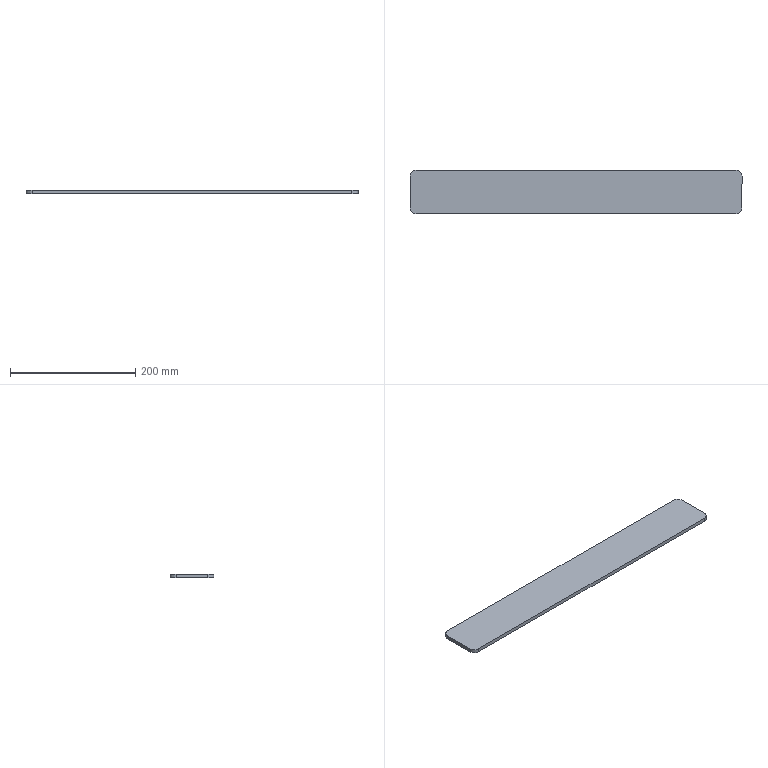Part | SolidWorks | features FlatPattern 1, SMBaseFlange 1, SheetMetal 1 | 1 solid | 10 faces | box 530 x 70 x 6 mm | volume 222085 mm3 | plane 6 | cylinder 4 | commonest cylinder face diameters 20 x4
STEP:
#1=CARTESIAN_POINT('',(430.,25.,0.));
#2=VERTEX_POINT('',#1);
#3=CARTESIAN_POINT('',(420.,35.,0.));
#4=VERTEX_POINT('',#3);
#5=CARTESIAN_POINT('',(420.,25.,0.));
#6=DIRECTION('',(0.,0.,1.));
#7=DIRECTION('',(1.,0.,0.));
#8=AXIS2_PLACEMENT_3D('',#5,#6,#7);
#9=CIRCLE('',#8,10.);
#10=EDGE_CURVE('',#2,#4,#9,.T.);
#11=ORIENTED_EDGE('',*,*,#10,.T.);
#12=CARTESIAN_POINT('',(420.,35.,6.));
#13=VERTEX_POINT('',#12);
#14=CARTESIAN_POINT('',(420.,35.,6.));
#15=DIRECTION('',(0.,0.,-1.));
#16=VECTOR('',#15,1000.);
#17=LINE('',#14,#16);
#18=EDGE_CURVE('',#13,#4,#17,.T.);
#19=ORIENTED_EDGE('',*,*,#18,.F.);
#20=CARTESIAN_POINT('',(430.,25.,6.));
#21=VERTEX_POINT('',#20);
#22=CARTESIAN_POINT('',(420.,25.,6.));
#23=DIRECTION('',(0.,0.,1.));
#24=DIRECTION('',(1.,0.,0.));
#25=AXIS2_PLACEMENT_3D('',#22,#23,#24);
#26=CIRCLE('',#25,10.);
#27=EDGE_CURVE('',#21,#13,#26,.T.);
#28=ORIENTED_EDGE('',*,*,#27,.F.);
#29=CARTESIAN_POINT('',(430.,25.,6.));
#30=DIRECTION('',(0.,0.,-1.));
#31=VECTOR('',#30,1000.);
#32=LINE('',#29,#31);
#33=EDGE_CURVE('',#21,#2,#32,.T.);
#34=ORIENTED_EDGE('',*,*,#33,.T.);
#35=EDGE_LOOP('',(#11,#19,#28,#34));
#36=FACE_OUTER_BOUND('',#35,.T.);
#37=CARTESIAN_POINT('',(420.,25.,6.));
#38=DIRECTION('',(0.,0.,-1.));
#39=DIRECTION('',(-1.,0.,0.));
#40=AXIS2_PLACEMENT_3D('',#37,#38,#39);
#41=CYLINDRICAL_SURFACE('',#40,10.);
#42=ADVANCED_FACE('',(#36),#41,.T.);
#43=CARTESIAN_POINT('',(-90.,35.,0.));
#44=VERTEX_POINT('',#43);
#45=CARTESIAN_POINT('',(420.,35.,0.));
#46=DIRECTION('',(-1.,0.,0.));
#47=VECTOR('',#46,1000.);
#48=LINE('',#45,#47);
#49=EDGE_CURVE('',#4,#44,#48,.T.);
#50=ORIENTED_EDGE('',*,*,#49,.T.);
#51=CARTESIAN_POINT('',(-90.,35.,6.));
#52=VERTEX_POINT('',#51);
#53=CARTESIAN_POINT('',(-90.,35.,6.));
#54=DIRECTION('',(0.,0.,-1.));
#55=VECTOR('',#54,1000.);
#56=LINE('',#53,#55);
#57=EDGE_CURVE('',#52,#44,#56,.T.);
#58=ORIENTED_EDGE('',*,*,#57,.F.);
#59=CARTESIAN_POINT('',(420.,35.,6.));
#60=DIRECTION('',(-1.,0.,0.));
#61=VECTOR('',#60,1000.);
#62=LINE('',#59,#61);
#63=EDGE_CURVE('',#13,#52,#62,.T.);
#64=ORIENTED_EDGE('',*,*,#63,.F.);
#65=ORIENTED_EDGE('',*,*,#18,.T.);
#66=EDGE_LOOP('',(#50,#58,#64,#65));
#67=FACE_OUTER_BOUND('',#66,.T.);
#68=CARTESIAN_POINT('',(420.,35.,6.));
#69=DIRECTION('',(0.,-1.,0.));
#70=DIRECTION('',(1.,0.,0.));
#71=AXIS2_PLACEMENT_3D('',#68,#69,#70);
#72=PLANE('',#71);
#73=ADVANCED_FACE('',(#67),#72,.F.);
#74=CARTESIAN_POINT('',(-100.,25.,0.));
#75=VERTEX_POINT('',#74);
#76=CARTESIAN_POINT('',(-90.,25.,0.));
#77=DIRECTION('',(0.,0.,1.));
#78=DIRECTION('',(1.,0.,0.));
#79=AXIS2_PLACEMENT_3D('',#76,#77,#78);
#80=CIRCLE('',#79,10.);
#81=EDGE_CURVE('',#44,#75,#80,.T.);
#82=ORIENTED_EDGE('',*,*,#81,.T.);
#83=CARTESIAN_POINT('',(-100.,25.,6.));
#84=VERTEX_POINT('',#83);
#85=CARTESIAN_POINT('',(-100.,25.,6.));
#86=DIRECTION('',(0.,0.,-1.));
#87=VECTOR('',#86,1000.);
#88=LINE('',#85,#87);
#89=EDGE_CURVE('',#84,#75,#88,.T.);
#90=ORIENTED_EDGE('',*,*,#89,.F.);
#91=CARTESIAN_POINT('',(-90.,25.,6.));
#92=DIRECTION('',(0.,0.,1.));
#93=DIRECTION('',(1.,0.,0.));
#94=AXIS2_PLACEMENT_3D('',#91,#92,#93);
#95=CIRCLE('',#94,10.);
#96=EDGE_CURVE('',#52,#84,#95,.T.);
#97=ORIENTED_EDGE('',*,*,#96,.F.);
#98=ORIENTED_EDGE('',*,*,#57,.T.);
#99=EDGE_LOOP('',(#82,#90,#97,#98));
#100=FACE_OUTER_BOUND('',#99,.T.);
#101=CARTESIAN_POINT('',(-90.,25.,6.));
#102=DIRECTION('',(0.,0.,-1.));
#103=DIRECTION('',(-1.,0.,0.));
#104=AXIS2_PLACEMENT_3D('',#101,#102,#103);
#105=CYLINDRICAL_SURFACE('',#104,10.);
#106=ADVANCED_FACE('',(#100),#105,.T.);
#107=CARTESIAN_POINT('',(-100.,-25.,0.));
#108=VERTEX_POINT('',#107);
#109=CARTESIAN_POINT('',(-100.,25.,0.));
#110=DIRECTION('',(0.,-1.,0.));
#111=VECTOR('',#110,1000.);
#112=LINE('',#109,#111);
#113=EDGE_CURVE('',#75,#108,#112,.T.);
#114=ORIENTED_EDGE('',*,*,#113,.T.);
#115=CARTESIAN_POINT('',(-100.,-25.,6.));
#116=VERTEX_POINT('',#115);
#117=CARTESIAN_POINT('',(-100.,-25.,6.));
#118=DIRECTION('',(0.,0.,-1.));
#119=VECTOR('',#118,1000.);
#120=LINE('',#117,#119);
#121=EDGE_CURVE('',#116,#108,#120,.T.);
#122=ORIENTED_EDGE('',*,*,#121,.F.);
#123=CARTESIAN_POINT('',(-100.,25.,6.));
#124=DIRECTION('',(0.,-1.,0.));
#125=VECTOR('',#124,1000.);
#126=LINE('',#123,#125);
#127=EDGE_CURVE('',#84,#116,#126,.T.);
#128=ORIENTED_EDGE('',*,*,#127,.F.);
#129=ORIENTED_EDGE('',*,*,#89,.T.);
#130=EDGE_LOOP('',(#114,#122,#128,#129));
#131=FACE_OUTER_BOUND('',#130,.T.);
#132=CARTESIAN_POINT('',(-100.,25.,6.));
#133=DIRECTION('',(1.,0.,0.));
#134=DIRECTION('',(0.,1.,0.));
#135=AXIS2_PLACEMENT_3D('',#132,#133,#134);
#136=PLANE('',#135);
#137=ADVANCED_FACE('',(#131),#136,.F.);
#138=CARTESIAN_POINT('',(-90.,-35.,0.));
#139=VERTEX_POINT('',#138);
#140=CARTESIAN_POINT('',(-90.,-25.,0.));
#141=DIRECTION('',(0.,0.,1.));
#142=DIRECTION('',(1.,0.,0.));
#143=AXIS2_PLACEMENT_3D('',#140,#141,#142);
#144=CIRCLE('',#143,10.);
#145=EDGE_CURVE('',#108,#139,#144,.T.);
#146=ORIENTED_EDGE('',*,*,#145,.T.);
#147=CARTESIAN_POINT('',(-90.,-35.,6.));
#148=VERTEX_POINT('',#147);
#149=CARTESIAN_POINT('',(-90.,-35.,6.));
#150=DIRECTION('',(0.,0.,-1.));
#151=VECTOR('',#150,1000.);
#152=LINE('',#149,#151);
#153=EDGE_CURVE('',#148,#139,#152,.T.);
#154=ORIENTED_EDGE('',*,*,#153,.F.);
#155=CARTESIAN_POINT('',(-90.,-25.,6.));
#156=DIRECTION('',(0.,0.,1.));
#157=DIRECTION('',(1.,0.,0.));
#158=AXIS2_PLACEMENT_3D('',#155,#156,#157);
#159=CIRCLE('',#158,10.);
#160=EDGE_CURVE('',#116,#148,#159,.T.);
#161=ORIENTED_EDGE('',*,*,#160,.F.);
#162=ORIENTED_EDGE('',*,*,#121,.T.);
#163=EDGE_LOOP('',(#146,#154,#161,#162));
#164=FACE_OUTER_BOUND('',#163,.T.);
#165=CARTESIAN_POINT('',(-90.,-25.,6.));
#166=DIRECTION('',(0.,0.,-1.));
#167=DIRECTION('',(-1.,0.,0.));
#168=AXIS2_PLACEMENT_3D('',#165,#166,#167);
#169=CYLINDRICAL_SURFACE('',#168,10.);
#170=ADVANCED_FACE('',(#164),#169,.T.);
#171=CARTESIAN_POINT('',(420.,-35.,0.));
#172=VERTEX_POINT('',#171);
#173=CARTESIAN_POINT('',(-90.,-35.,0.));
#174=DIRECTION('',(1.,0.,0.));
#175=VECTOR('',#174,1000.);
#176=LINE('',#173,#175);
#177=EDGE_CURVE('',#139,#172,#176,.T.);
#178=ORIENTED_EDGE('',*,*,#177,.T.);
#179=CARTESIAN_POINT('',(420.,-35.,6.));
#180=VERTEX_POINT('',#179);
#181=CARTESIAN_POINT('',(420.,-35.,6.));
#182=DIRECTION('',(0.,0.,-1.));
#183=VECTOR('',#182,1000.);
#184=LINE('',#181,#183);
#185=EDGE_CURVE('',#180,#172,#184,.T.);
#186=ORIENTED_EDGE('',*,*,#185,.F.);
#187=CARTESIAN_POINT('',(-90.,-35.,6.));
#188=DIRECTION('',(1.,0.,0.));
#189=VECTOR('',#188,1000.);
#190=LINE('',#187,#189);
#191=EDGE_CURVE('',#148,#180,#190,.T.);
#192=ORIENTED_EDGE('',*,*,#191,.F.);
#193=ORIENTED_EDGE('',*,*,#153,.T.);
#194=EDGE_LOOP('',(#178,#186,#192,#193));
#195=FACE_OUTER_BOUND('',#194,.T.);
#196=CARTESIAN_POINT('',(-90.,-35.,6.));
#197=DIRECTION('',(0.,1.,0.));
#198=DIRECTION('',(-1.,0.,0.));
#199=AXIS2_PLACEMENT_3D('',#196,#197,#198);
#200=PLANE('',#199);
#201=ADVANCED_FACE('',(#195),#200,.F.);
#202=CARTESIAN_POINT('',(430.,-25.,0.));
#203=VERTEX_POINT('',#202);
#204=CARTESIAN_POINT('',(420.,-25.,0.));
#205=DIRECTION('',(0.,0.,1.));
#206=DIRECTION('',(-1.,0.,0.));
#207=AXIS2_PLACEMENT_3D('',#204,#205,#206);
#208=CIRCLE('',#207,10.);
#209=EDGE_CURVE('',#172,#203,#208,.T.);
#210=ORIENTED_EDGE('',*,*,#209,.T.);
#211=CARTESIAN_POINT('',(430.,-25.,6.));
#212=VERTEX_POINT('',#211);
#213=CARTESIAN_POINT('',(430.,-25.,6.));
#214=DIRECTION('',(0.,0.,-1.));
#215=VECTOR('',#214,1000.);
#216=LINE('',#213,#215);
#217=EDGE_CURVE('',#212,#203,#216,.T.);
#218=ORIENTED_EDGE('',*,*,#217,.F.);
#219=CARTESIAN_POINT('',(420.,-25.,6.));
#220=DIRECTION('',(0.,0.,1.));
#221=DIRECTION('',(-1.,0.,0.));
#222=AXIS2_PLACEMENT_3D('',#219,#220,#221);
#223=CIRCLE('',#222,10.);
#224=EDGE_CURVE('',#180,#212,#223,.T.);
#225=ORIENTED_EDGE('',*,*,#224,.F.);
#226=ORIENTED_EDGE('',*,*,#185,.T.);
#227=EDGE_LOOP('',(#210,#218,#225,#226));
#228=FACE_OUTER_BOUND('',#227,.T.);
#229=CARTESIAN_POINT('',(420.,-25.,6.));
#230=DIRECTION('',(0.,0.,-1.));
#231=DIRECTION('',(-1.,0.,0.));
#232=AXIS2_PLACEMENT_3D('',#229,#230,#231);
#233=CYLINDRICAL_SURFACE('',#232,10.);
#234=ADVANCED_FACE('',(#228),#233,.T.);
#235=CARTESIAN_POINT('',(430.,-25.,0.));
#236=DIRECTION('',(0.,1.,0.));
#237=VECTOR('',#236,1000.);
#238=LINE('',#235,#237);
#239=EDGE_CURVE('',#203,#2,#238,.T.);
#240=ORIENTED_EDGE('',*,*,#239,.T.);
#241=ORIENTED_EDGE('',*,*,#33,.F.);
#242=CARTESIAN_POINT('',(430.,-25.,6.));
#243=DIRECTION('',(0.,1.,0.));
#244=VECTOR('',#243,1000.);
#245=LINE('',#242,#244);
#246=EDGE_CURVE('',#212,#21,#245,.T.);
#247=ORIENTED_EDGE('',*,*,#246,.F.);
#248=ORIENTED_EDGE('',*,*,#217,.T.);
#249=EDGE_LOOP('',(#240,#241,#247,#248));
#250=FACE_OUTER_BOUND('',#249,.T.);
#251=CARTESIAN_POINT('',(430.,-25.,6.));
#252=DIRECTION('',(-1.,0.,0.));
#253=DIRECTION('',(0.,-1.,0.));
#254=AXIS2_PLACEMENT_3D('',#251,#252,#253);
#255=PLANE('',#254);
#256=ADVANCED_FACE('',(#250),#255,.F.);
#257=ORIENTED_EDGE('',*,*,#27,.T.);
#258=ORIENTED_EDGE('',*,*,#63,.T.);
#259=ORIENTED_EDGE('',*,*,#96,.T.);
#260=ORIENTED_EDGE('',*,*,#127,.T.);
#261=ORIENTED_EDGE('',*,*,#160,.T.);
#262=ORIENTED_EDGE('',*,*,#191,.T.);
#263=ORIENTED_EDGE('',*,*,#224,.T.);
#264=ORIENTED_EDGE('',*,*,#246,.T.);
#265=EDGE_LOOP('',(#257,#258,#259,#260,#261,#262,#263,#264));
#266=FACE_OUTER_BOUND('',#265,.T.);
#267=CARTESIAN_POINT('',(420.,25.,6.));
#268=DIRECTION('',(0.,0.,1.));
#269=DIRECTION('',(1.,0.,0.));
#270=AXIS2_PLACEMENT_3D('',#267,#268,#269);
#271=PLANE('',#270);
#272=ADVANCED_FACE('',(#266),#271,.T.);
#273=ORIENTED_EDGE('',*,*,#10,.F.);
#274=ORIENTED_EDGE('',*,*,#239,.F.);
#275=ORIENTED_EDGE('',*,*,#209,.F.);
#276=ORIENTED_EDGE('',*,*,#177,.F.);
#277=ORIENTED_EDGE('',*,*,#145,.F.);
#278=ORIENTED_EDGE('',*,*,#113,.F.);
#279=ORIENTED_EDGE('',*,*,#81,.F.);
#280=ORIENTED_EDGE('',*,*,#49,.F.);
#281=EDGE_LOOP('',(#273,#274,#275,#276,#277,#278,#279,#280));
#282=FACE_OUTER_BOUND('',#281,.T.);
#283=CARTESIAN_POINT('',(420.,25.,0.));
#284=DIRECTION('',(0.,0.,1.));
#285=DIRECTION('',(1.,0.,0.));
#286=AXIS2_PLACEMENT_3D('',#283,#284,#285);
#287=PLANE('',#286);
#288=ADVANCED_FACE('',(#282),#287,.F.);
#289=CLOSED_SHELL('',(#42,#73,#106,#137,#170,#201,#234,#256,#272,#288));
#290=MANIFOLD_SOLID_BREP('',#289);
#291=CARTESIAN_POINT('',(0.,0.,0.));
#292=DIRECTION('',(0.,0.,1.));
#293=DIRECTION('',(1.,0.,0.));
#294=AXIS2_PLACEMENT_3D('',#291,#292,#293);
#295=(LENGTH_UNIT()NAMED_UNIT(*)SI_UNIT(.MILLI.,.METRE.));
#296=UNCERTAINTY_MEASURE_WITH_UNIT(LENGTH_MEASURE(0.00001),#295,'','');
#297=(NAMED_UNIT(*)PLANE_ANGLE_UNIT()SI_UNIT($,.RADIAN.));
#298=(NAMED_UNIT(*)SI_UNIT($,.STERADIAN.)SOLID_ANGLE_UNIT());
#299=(GEOMETRIC_REPRESENTATION_CONTEXT(3)GLOBAL_UNCERTAINTY_ASSIGNED_CONTEXT((#296))GLOBAL_UNIT_ASSIGNED_CONTEXT((#295,#297,#298))REPRESENTATION_CONTEXT('',''));
#300=ADVANCED_BREP_SHAPE_REPRESENTATION('',(#290,#294),#299);